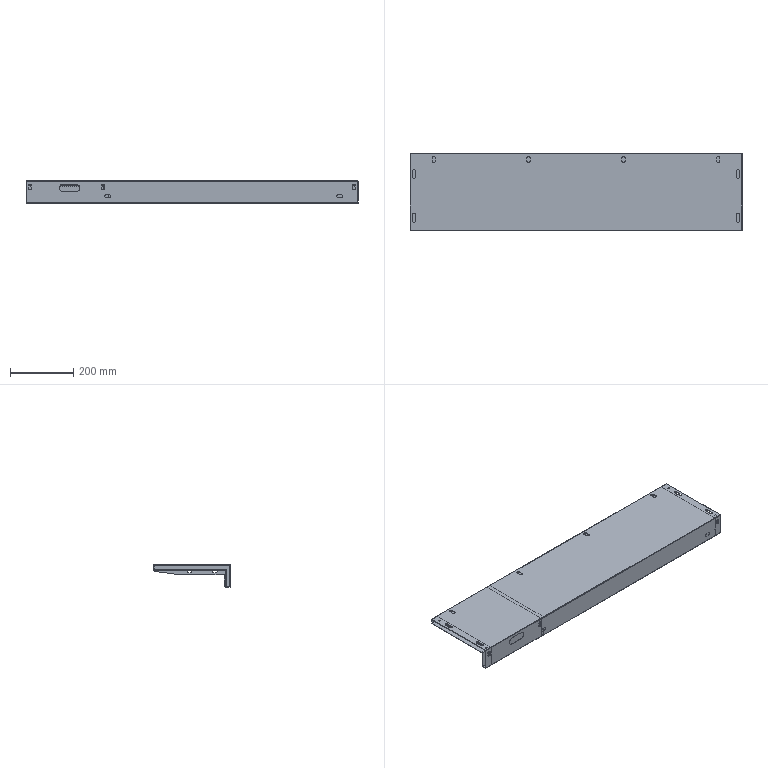Part | 5 solids | 288 faces | box 1050 x 243.5 x 70 mm | volume 757846 mm3 | plane 169 | cylinder 119 | commonest cylinder face diameters 6 x46 10 x24 9 x20 0.4 x8 11 x8 2.4 x5